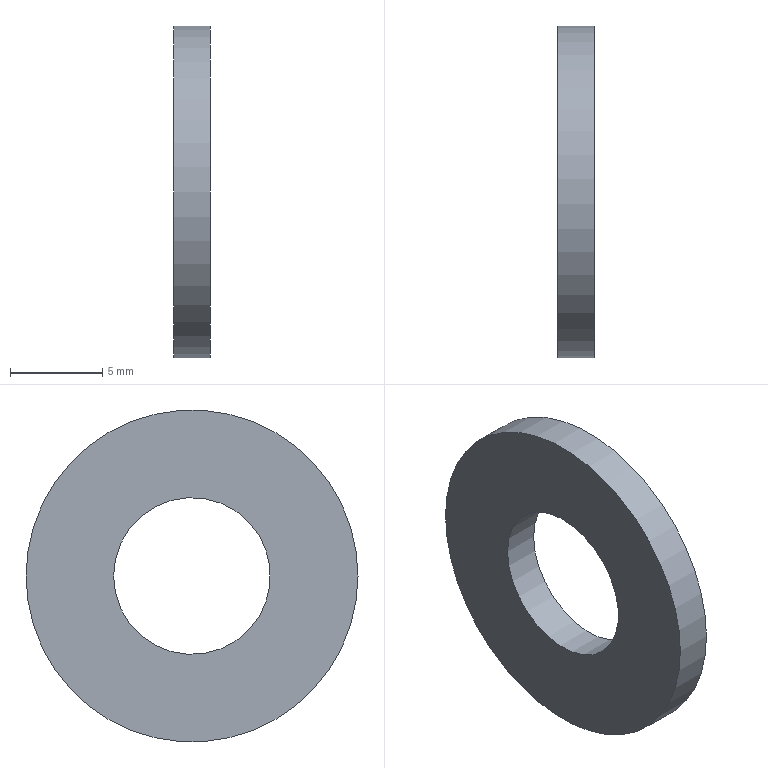Part | NX | 1 solid | 4 faces | box 2 x 18 x 18 mm | volume 395.448 mm3 | cylinder 2 | plane 2 | commonest cylinder face diameters 8.5 x1 18 x1
STEP:
#1=CARTESIAN_POINT('',(2.,9.,0.));
#2=VERTEX_POINT('',#1);
#3=CARTESIAN_POINT('',(2.,0.,0.));
#4=DIRECTION('',(1.,0.,0.));
#5=DIRECTION('',(0.,1.,0.));
#6=AXIS2_PLACEMENT_3D('',#3,#4,#5);
#7=CIRCLE('',#6,9.);
#8=EDGE_CURVE('',#2,#2,#7,.T.);
#9=ORIENTED_EDGE('',*,*,#8,.F.);
#10=EDGE_LOOP('',(#9));
#11=FACE_BOUND('',#10,.T.);
#12=CARTESIAN_POINT('',(0.,9.,0.));
#13=VERTEX_POINT('',#12);
#14=CARTESIAN_POINT('',(0.,0.,0.));
#15=DIRECTION('',(1.,0.,0.));
#16=DIRECTION('',(0.,1.,0.));
#17=AXIS2_PLACEMENT_3D('',#14,#15,#16);
#18=CIRCLE('',#17,9.);
#19=EDGE_CURVE('',#13,#13,#18,.T.);
#20=ORIENTED_EDGE('',*,*,#19,.T.);
#21=EDGE_LOOP('',(#20));
#22=FACE_BOUND('',#21,.T.);
#23=CARTESIAN_POINT('',(2.,0.,0.));
#24=DIRECTION('',(-1.,0.,0.));
#25=DIRECTION('',(0.,0.,-1.));
#26=AXIS2_PLACEMENT_3D('',#23,#24,#25);
#27=CYLINDRICAL_SURFACE('',#26,9.);
#28=ADVANCED_FACE('',(#11,#22),#27,.T.);
#29=CARTESIAN_POINT('',(2.,4.25,0.));
#30=VERTEX_POINT('',#29);
#31=CARTESIAN_POINT('',(2.,0.,0.));
#32=DIRECTION('',(1.,0.,0.));
#33=DIRECTION('',(0.,1.,0.));
#34=AXIS2_PLACEMENT_3D('',#31,#32,#33);
#35=CIRCLE('',#34,4.25);
#36=EDGE_CURVE('',#30,#30,#35,.T.);
#37=ORIENTED_EDGE('',*,*,#36,.T.);
#38=EDGE_LOOP('',(#37));
#39=FACE_BOUND('',#38,.T.);
#40=CARTESIAN_POINT('',(0.,4.25,0.));
#41=VERTEX_POINT('',#40);
#42=CARTESIAN_POINT('',(0.,0.,0.));
#43=DIRECTION('',(1.,0.,0.));
#44=DIRECTION('',(0.,1.,0.));
#45=AXIS2_PLACEMENT_3D('',#42,#43,#44);
#46=CIRCLE('',#45,4.25);
#47=EDGE_CURVE('',#41,#41,#46,.T.);
#48=ORIENTED_EDGE('',*,*,#47,.F.);
#49=EDGE_LOOP('',(#48));
#50=FACE_BOUND('',#49,.T.);
#51=CARTESIAN_POINT('',(2.,0.,0.));
#52=DIRECTION('',(-1.,0.,0.));
#53=DIRECTION('',(0.,0.,-1.));
#54=AXIS2_PLACEMENT_3D('',#51,#52,#53);
#55=CYLINDRICAL_SURFACE('',#54,4.25);
#56=ADVANCED_FACE('',(#39,#50),#55,.F.);
#57=ORIENTED_EDGE('',*,*,#8,.T.);
#58=EDGE_LOOP('',(#57));
#59=FACE_BOUND('',#58,.T.);
#60=ORIENTED_EDGE('',*,*,#36,.F.);
#61=EDGE_LOOP('',(#60));
#62=FACE_BOUND('',#61,.T.);
#63=CARTESIAN_POINT('',(2.,0.,0.));
#64=DIRECTION('',(1.,0.,0.));
#65=DIRECTION('',(0.,0.,1.));
#66=AXIS2_PLACEMENT_3D('',#63,#64,#65);
#67=PLANE('',#66);
#68=ADVANCED_FACE('',(#59,#62),#67,.T.);
#69=ORIENTED_EDGE('',*,*,#19,.F.);
#70=EDGE_LOOP('',(#69));
#71=FACE_BOUND('',#70,.T.);
#72=ORIENTED_EDGE('',*,*,#47,.T.);
#73=EDGE_LOOP('',(#72));
#74=FACE_BOUND('',#73,.T.);
#75=CARTESIAN_POINT('',(0.,0.,0.));
#76=DIRECTION('',(1.,0.,0.));
#77=DIRECTION('',(0.,0.,1.));
#78=AXIS2_PLACEMENT_3D('',#75,#76,#77);
#79=PLANE('',#78);
#80=ADVANCED_FACE('',(#71,#74),#79,.F.);
#81=CLOSED_SHELL('',(#28,#56,#68,#80));
#82=MANIFOLD_SOLID_BREP('',#81);
#83=(LENGTH_UNIT()NAMED_UNIT(*)SI_UNIT(.MILLI.,.METRE.));
#84=UNCERTAINTY_MEASURE_WITH_UNIT(LENGTH_MEASURE(0.00002),#83,'','');
#85=(NAMED_UNIT(*)PLANE_ANGLE_UNIT()SI_UNIT($,.RADIAN.));
#86=PLANE_ANGLE_MEASURE_WITH_UNIT(PLANE_ANGLE_MEASURE(0.01745),#85);
#87=DIMENSIONAL_EXPONENTS(0.,0.,0.,0.,0.,0.,0.);
#88=(CONVERSION_BASED_UNIT('DEGREE',#86)NAMED_UNIT(#87)PLANE_ANGLE_UNIT());
#89=(NAMED_UNIT(*)SI_UNIT($,.STERADIAN.)SOLID_ANGLE_UNIT());
#90=(GEOMETRIC_REPRESENTATION_CONTEXT(3)GLOBAL_UNCERTAINTY_ASSIGNED_CONTEXT((#84))GLOBAL_UNIT_ASSIGNED_CONTEXT((#83,#88,#89))REPRESENTATION_CONTEXT('',''));
#91=ADVANCED_BREP_SHAPE_REPRESENTATION('',(#82),#90);